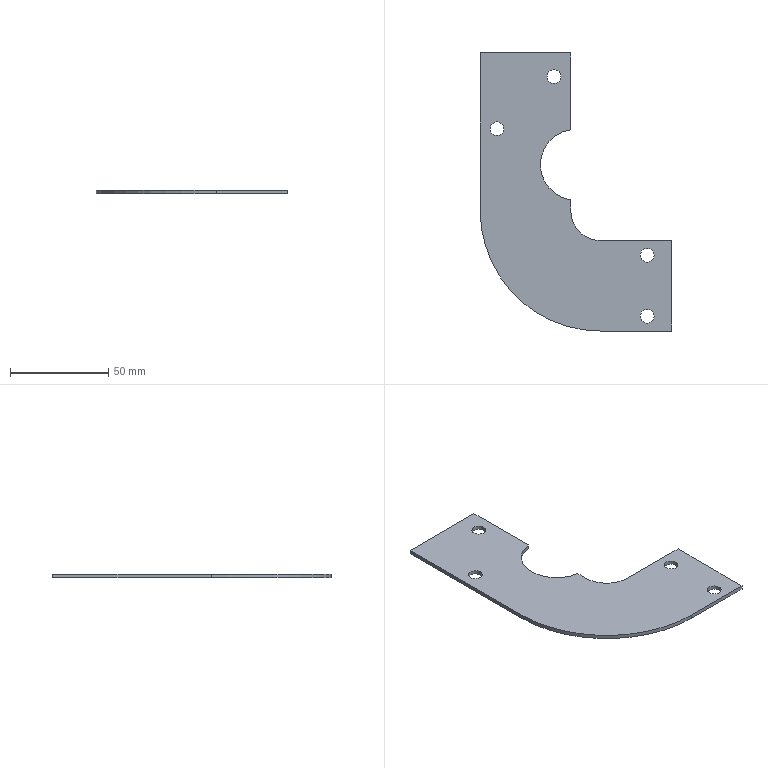Part | STEP file | 1_id1250_x_t | 1 solid | 20 faces | box 97.332 x 141.374 x 2 mm | volume 15084 mm3 | cylinder 11 | plane 9 | commonest cylinder face diameters 7 x8 30 x1 36 x1 122 x1